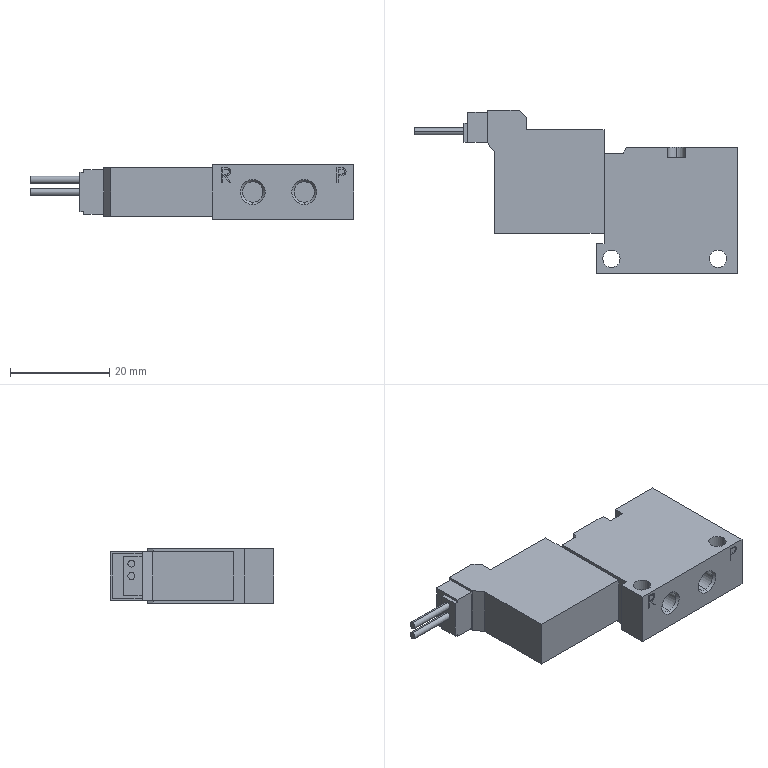Part | SolidWorks | features ICE 2, BaseBody 1 | 1 solid | 146 faces | box 65.3 x 33 x 11 mm | volume 11908 mm3 | plane 88 | cylinder 29 | spline 21 | cone 8 | commonest cylinder face diameters 4.13 x8 3.5 x7 1.4 x4 2.4 x4 3.1 x2 8.8 x2